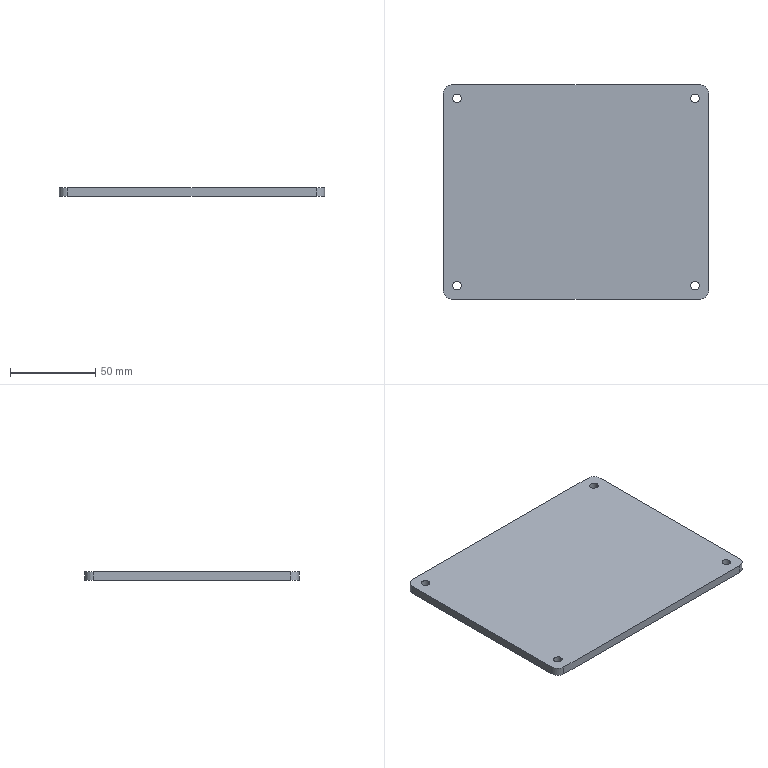Part | STEP file | Wrench controller display guard | 1 solid | 18 faces | box 156 x 126 x 5 mm | volume 97780 mm3 | cylinder 12 | plane 6 | commonest cylinder face diameters 5 x8 10 x4
STEP:
#1=CARTESIAN_POINT('',(0.,0.,0.));
#2=DIRECTION('',(0.,0.,1.));
#3=DIRECTION('',(1.,0.,0.));
#4=AXIS2_PLACEMENT_3D('',#1,#2,#3);
#5=CARTESIAN_POINT('',(67.5,-55.,5.));
#6=VERTEX_POINT('',#5);
#7=CARTESIAN_POINT('',(67.5,-55.,0.));
#8=VERTEX_POINT('',#7);
#9=CARTESIAN_POINT('',(67.5,-55.,5.));
#10=DIRECTION('',(0.,0.,-1.));
#11=VECTOR('',#10,1.);
#12=LINE('',#9,#11);
#13=CARTESIAN_POINT('',(70.,-55.,5.));
#14=DIRECTION('',(0.,0.,-1.));
#15=DIRECTION('',(-1.,0.,0.));
#16=AXIS2_PLACEMENT_3D('',#13,#14,#15);
#17=CYLINDRICAL_SURFACE('',#16,2.5);
#18=CARTESIAN_POINT('',(6.283,0.));
#19=DIRECTION('',(0.,1.));
#20=VECTOR('',#19,1.);
#21=LINE('',#18,#20);
#22=(GEOMETRIC_REPRESENTATION_CONTEXT(2)PARAMETRIC_REPRESENTATION_CONTEXT()REPRESENTATION_CONTEXT('',''));
#23=DEFINITIONAL_REPRESENTATION('',(#21),#22);
#24=PCURVE('',#17,#23);
#25=CARTESIAN_POINT('',(70.,-55.,5.));
#26=DIRECTION('',(0.,0.,-1.));
#27=DIRECTION('',(-1.,0.,0.));
#28=AXIS2_PLACEMENT_3D('',#25,#26,#27);
#29=CYLINDRICAL_SURFACE('',#28,2.5);
#30=CARTESIAN_POINT('',(0.,0.));
#31=DIRECTION('',(0.,1.));
#32=VECTOR('',#31,1.);
#33=LINE('',#30,#32);
#34=(GEOMETRIC_REPRESENTATION_CONTEXT(2)PARAMETRIC_REPRESENTATION_CONTEXT()REPRESENTATION_CONTEXT('',''));
#35=DEFINITIONAL_REPRESENTATION('',(#33),#34);
#36=PCURVE('',#29,#35);
#37=SURFACE_CURVE('',#12,(#24,#36),.PCURVE_S1.);
#38=EDGE_CURVE('',#6,#8,#37,.T.);
#39=ORIENTED_EDGE('',*,*,#38,.T.);
#40=CARTESIAN_POINT('',(72.5,-55.,0.));
#41=VERTEX_POINT('',#40);
#42=CARTESIAN_POINT('',(70.,-55.,0.));
#43=DIRECTION('',(0.,0.,1.));
#44=DIRECTION('',(-1.,0.,0.));
#45=AXIS2_PLACEMENT_3D('',#42,#43,#44);
#46=CIRCLE('',#45,2.5);
#47=CARTESIAN_POINT('',(6.283,5.));
#48=DIRECTION('',(-1.,0.));
#49=VECTOR('',#48,1.);
#50=LINE('',#47,#49);
#51=(GEOMETRIC_REPRESENTATION_CONTEXT(2)PARAMETRIC_REPRESENTATION_CONTEXT()REPRESENTATION_CONTEXT('',''));
#52=DEFINITIONAL_REPRESENTATION('',(#50),#51);
#53=PCURVE('',#17,#52);
#54=CARTESIAN_POINT('',(73.,-58.,0.));
#55=DIRECTION('',(0.,0.,1.));
#56=DIRECTION('',(1.,0.,0.));
#57=AXIS2_PLACEMENT_3D('',#54,#55,#56);
#58=PLANE('',#57);
#59=CARTESIAN_POINT('',(-3.,3.));
#60=DIRECTION('',(-1.,0.));
#61=AXIS2_PLACEMENT_2D('',#59,#60);
#62=CIRCLE('',#61,2.5);
#63=(GEOMETRIC_REPRESENTATION_CONTEXT(2)PARAMETRIC_REPRESENTATION_CONTEXT()REPRESENTATION_CONTEXT('',''));
#64=DEFINITIONAL_REPRESENTATION('',(#62),#63);
#65=PCURVE('',#58,#64);
#66=SURFACE_CURVE('',#46,(#53,#65),.PCURVE_S1.);
#67=EDGE_CURVE('',#8,#41,#66,.T.);
#68=ORIENTED_EDGE('',*,*,#67,.T.);
#69=CARTESIAN_POINT('',(72.5,-55.,5.));
#70=VERTEX_POINT('',#69);
#71=CARTESIAN_POINT('',(72.5,-55.,5.));
#72=DIRECTION('',(0.,0.,-1.));
#73=VECTOR('',#72,1.);
#74=LINE('',#71,#73);
#75=CARTESIAN_POINT('',(3.142,0.));
#76=DIRECTION('',(0.,1.));
#77=VECTOR('',#76,1.);
#78=LINE('',#75,#77);
#79=(GEOMETRIC_REPRESENTATION_CONTEXT(2)PARAMETRIC_REPRESENTATION_CONTEXT()REPRESENTATION_CONTEXT('',''));
#80=DEFINITIONAL_REPRESENTATION('',(#78),#79);
#81=PCURVE('',#17,#80);
#82=CARTESIAN_POINT('',(3.142,0.));
#83=DIRECTION('',(0.,1.));
#84=VECTOR('',#83,1.);
#85=LINE('',#82,#84);
#86=(GEOMETRIC_REPRESENTATION_CONTEXT(2)PARAMETRIC_REPRESENTATION_CONTEXT()REPRESENTATION_CONTEXT('',''));
#87=DEFINITIONAL_REPRESENTATION('',(#85),#86);
#88=PCURVE('',#29,#87);
#89=SURFACE_CURVE('',#74,(#81,#88),.PCURVE_S1.);
#90=EDGE_CURVE('',#70,#41,#89,.T.);
#91=ORIENTED_EDGE('',*,*,#90,.F.);
#92=CARTESIAN_POINT('',(70.,-55.,5.));
#93=DIRECTION('',(0.,0.,-1.));
#94=DIRECTION('',(-1.,0.,0.));
#95=AXIS2_PLACEMENT_3D('',#92,#93,#94);
#96=CIRCLE('',#95,2.5);
#97=CARTESIAN_POINT('',(0.,0.));
#98=DIRECTION('',(1.,0.));
#99=VECTOR('',#98,1.);
#100=LINE('',#97,#99);
#101=(GEOMETRIC_REPRESENTATION_CONTEXT(2)PARAMETRIC_REPRESENTATION_CONTEXT()REPRESENTATION_CONTEXT('',''));
#102=DEFINITIONAL_REPRESENTATION('',(#100),#101);
#103=PCURVE('',#17,#102);
#104=CARTESIAN_POINT('',(73.,-58.,5.));
#105=DIRECTION('',(0.,0.,1.));
#106=DIRECTION('',(1.,0.,0.));
#107=AXIS2_PLACEMENT_3D('',#104,#105,#106);
#108=PLANE('',#107);
#109=CARTESIAN_POINT('',(-5.5,3.));
#110=CARTESIAN_POINT('',(-5.5,7.33));
#111=CARTESIAN_POINT('',(-1.75,5.165));
#112=CARTESIAN_POINT('',(2.,3.));
#113=CARTESIAN_POINT('',(-1.75,0.8349));
#114=CARTESIAN_POINT('',(-5.5,-1.33));
#115=CARTESIAN_POINT('',(-5.5,3.));
#116=(BOUNDED_CURVE()B_SPLINE_CURVE(2,(#109,#110,#111,#112,#113,#114,#115),.UNSPECIFIED.,.T.,.F.)B_SPLINE_CURVE_WITH_KNOTS((1,2,2,2,2,1),(-2.094,0.,2.094,4.189,6.283,8.378),.UNSPECIFIED.)CURVE()GEOMETRIC_REPRESENTATION_ITEM()RATIONAL_B_SPLINE_CURVE((1.,0.5,1.,0.5,1.,0.5,1.))REPRESENTATION_ITEM(''));
#117=(GEOMETRIC_REPRESENTATION_CONTEXT(2)PARAMETRIC_REPRESENTATION_CONTEXT()REPRESENTATION_CONTEXT('',''));
#118=DEFINITIONAL_REPRESENTATION('',(#116),#117);
#119=PCURVE('',#108,#118);
#120=SURFACE_CURVE('',#96,(#103,#119),.PCURVE_S1.);
#121=EDGE_CURVE('',#70,#6,#120,.T.);
#122=ORIENTED_EDGE('',*,*,#121,.T.);
#123=EDGE_LOOP('',(#39,#68,#91,#122));
#124=FACE_BOUND('',#123,.F.);
#125=ADVANCED_FACE('',(#124),#17,.F.);
#126=CARTESIAN_POINT('',(67.5,55.,5.));
#127=VERTEX_POINT('',#126);
#128=CARTESIAN_POINT('',(67.5,55.,0.));
#129=VERTEX_POINT('',#128);
#130=CARTESIAN_POINT('',(67.5,55.,5.));
#131=DIRECTION('',(0.,0.,-1.));
#132=VECTOR('',#131,1.);
#133=LINE('',#130,#132);
#134=CARTESIAN_POINT('',(70.,55.,5.));
#135=DIRECTION('',(0.,0.,-1.));
#136=DIRECTION('',(-1.,0.,0.));
#137=AXIS2_PLACEMENT_3D('',#134,#135,#136);
#138=CYLINDRICAL_SURFACE('',#137,2.5);
#139=CARTESIAN_POINT('',(6.283,0.));
#140=DIRECTION('',(0.,1.));
#141=VECTOR('',#140,1.);
#142=LINE('',#139,#141);
#143=(GEOMETRIC_REPRESENTATION_CONTEXT(2)PARAMETRIC_REPRESENTATION_CONTEXT()REPRESENTATION_CONTEXT('',''));
#144=DEFINITIONAL_REPRESENTATION('',(#142),#143);
#145=PCURVE('',#138,#144);
#146=CARTESIAN_POINT('',(70.,55.,5.));
#147=DIRECTION('',(0.,0.,-1.));
#148=DIRECTION('',(-1.,0.,0.));
#149=AXIS2_PLACEMENT_3D('',#146,#147,#148);
#150=CYLINDRICAL_SURFACE('',#149,2.5);
#151=CARTESIAN_POINT('',(0.,0.));
#152=DIRECTION('',(0.,1.));
#153=VECTOR('',#152,1.);
#154=LINE('',#151,#153);
#155=(GEOMETRIC_REPRESENTATION_CONTEXT(2)PARAMETRIC_REPRESENTATION_CONTEXT()REPRESENTATION_CONTEXT('',''));
#156=DEFINITIONAL_REPRESENTATION('',(#154),#155);
#157=PCURVE('',#150,#156);
#158=SURFACE_CURVE('',#133,(#145,#157),.PCURVE_S1.);
#159=EDGE_CURVE('',#127,#129,#158,.T.);
#160=ORIENTED_EDGE('',*,*,#159,.T.);
#161=CARTESIAN_POINT('',(72.5,55.,0.));
#162=VERTEX_POINT('',#161);
#163=CARTESIAN_POINT('',(70.,55.,0.));
#164=DIRECTION('',(0.,0.,1.));
#165=DIRECTION('',(-1.,0.,0.));
#166=AXIS2_PLACEMENT_3D('',#163,#164,#165);
#167=CIRCLE('',#166,2.5);
#168=CARTESIAN_POINT('',(6.283,5.));
#169=DIRECTION('',(-1.,0.));
#170=VECTOR('',#169,1.);
#171=LINE('',#168,#170);
#172=(GEOMETRIC_REPRESENTATION_CONTEXT(2)PARAMETRIC_REPRESENTATION_CONTEXT()REPRESENTATION_CONTEXT('',''));
#173=DEFINITIONAL_REPRESENTATION('',(#171),#172);
#174=PCURVE('',#138,#173);
#175=CARTESIAN_POINT('',(-3.,113.));
#176=DIRECTION('',(-1.,0.));
#177=AXIS2_PLACEMENT_2D('',#175,#176);
#178=CIRCLE('',#177,2.5);
#179=(GEOMETRIC_REPRESENTATION_CONTEXT(2)PARAMETRIC_REPRESENTATION_CONTEXT()REPRESENTATION_CONTEXT('',''));
#180=DEFINITIONAL_REPRESENTATION('',(#178),#179);
#181=PCURVE('',#58,#180);
#182=SURFACE_CURVE('',#167,(#174,#181),.PCURVE_S1.);
#183=EDGE_CURVE('',#129,#162,#182,.T.);
#184=ORIENTED_EDGE('',*,*,#183,.T.);
#185=CARTESIAN_POINT('',(72.5,55.,5.));
#186=VERTEX_POINT('',#185);
#187=CARTESIAN_POINT('',(72.5,55.,5.));
#188=DIRECTION('',(0.,0.,-1.));
#189=VECTOR('',#188,1.);
#190=LINE('',#187,#189);
#191=CARTESIAN_POINT('',(3.142,0.));
#192=DIRECTION('',(0.,1.));
#193=VECTOR('',#192,1.);
#194=LINE('',#191,#193);
#195=(GEOMETRIC_REPRESENTATION_CONTEXT(2)PARAMETRIC_REPRESENTATION_CONTEXT()REPRESENTATION_CONTEXT('',''));
#196=DEFINITIONAL_REPRESENTATION('',(#194),#195);
#197=PCURVE('',#138,#196);
#198=CARTESIAN_POINT('',(3.142,0.));
#199=DIRECTION('',(0.,1.));
#200=VECTOR('',#199,1.);
#201=LINE('',#198,#200);
#202=(GEOMETRIC_REPRESENTATION_CONTEXT(2)PARAMETRIC_REPRESENTATION_CONTEXT()REPRESENTATION_CONTEXT('',''));
#203=DEFINITIONAL_REPRESENTATION('',(#201),#202);
#204=PCURVE('',#150,#203);
#205=SURFACE_CURVE('',#190,(#197,#204),.PCURVE_S1.);
#206=EDGE_CURVE('',#186,#162,#205,.T.);
#207=ORIENTED_EDGE('',*,*,#206,.F.);
#208=CARTESIAN_POINT('',(70.,55.,5.));
#209=DIRECTION('',(0.,0.,-1.));
#210=DIRECTION('',(-1.,0.,0.));
#211=AXIS2_PLACEMENT_3D('',#208,#209,#210);
#212=CIRCLE('',#211,2.5);
#213=CARTESIAN_POINT('',(0.,0.));
#214=DIRECTION('',(1.,0.));
#215=VECTOR('',#214,1.);
#216=LINE('',#213,#215);
#217=(GEOMETRIC_REPRESENTATION_CONTEXT(2)PARAMETRIC_REPRESENTATION_CONTEXT()REPRESENTATION_CONTEXT('',''));
#218=DEFINITIONAL_REPRESENTATION('',(#216),#217);
#219=PCURVE('',#138,#218);
#220=CARTESIAN_POINT('',(-5.5,113.));
#221=CARTESIAN_POINT('',(-5.5,117.33));
#222=CARTESIAN_POINT('',(-1.75,115.165));
#223=CARTESIAN_POINT('',(2.,113.));
#224=CARTESIAN_POINT('',(-1.75,110.835));
#225=CARTESIAN_POINT('',(-5.5,108.67));
#226=CARTESIAN_POINT('',(-5.5,113.));
#227=(BOUNDED_CURVE()B_SPLINE_CURVE(2,(#220,#221,#222,#223,#224,#225,#226),.UNSPECIFIED.,.T.,.F.)B_SPLINE_CURVE_WITH_KNOTS((1,2,2,2,2,1),(-2.094,0.,2.094,4.189,6.283,8.378),.UNSPECIFIED.)CURVE()GEOMETRIC_REPRESENTATION_ITEM()RATIONAL_B_SPLINE_CURVE((1.,0.5,1.,0.5,1.,0.5,1.))REPRESENTATION_ITEM(''));
#228=(GEOMETRIC_REPRESENTATION_CONTEXT(2)PARAMETRIC_REPRESENTATION_CONTEXT()REPRESENTATION_CONTEXT('',''));
#229=DEFINITIONAL_REPRESENTATION('',(#227),#228);
#230=PCURVE('',#108,#229);
#231=SURFACE_CURVE('',#212,(#219,#230),.PCURVE_S1.);
#232=EDGE_CURVE('',#186,#127,#231,.T.);
#233=ORIENTED_EDGE('',*,*,#232,.T.);
#234=EDGE_LOOP('',(#160,#184,#207,#233));
#235=FACE_BOUND('',#234,.F.);
#236=ADVANCED_FACE('',(#235),#138,.F.);
#237=CARTESIAN_POINT('',(-72.5,55.,5.));
#238=VERTEX_POINT('',#237);
#239=CARTESIAN_POINT('',(-72.5,55.,0.));
#240=VERTEX_POINT('',#239);
#241=CARTESIAN_POINT('',(-72.5,55.,5.));
#242=DIRECTION('',(0.,0.,-1.));
#243=VECTOR('',#242,1.);
#244=LINE('',#241,#243);
#245=CARTESIAN_POINT('',(-70.,55.,5.));
#246=DIRECTION('',(0.,0.,-1.));
#247=DIRECTION('',(-1.,0.,0.));
#248=AXIS2_PLACEMENT_3D('',#245,#246,#247);
#249=CYLINDRICAL_SURFACE('',#248,2.5);
#250=CARTESIAN_POINT('',(6.283,0.));
#251=DIRECTION('',(0.,1.));
#252=VECTOR('',#251,1.);
#253=LINE('',#250,#252);
#254=(GEOMETRIC_REPRESENTATION_CONTEXT(2)PARAMETRIC_REPRESENTATION_CONTEXT()REPRESENTATION_CONTEXT('',''));
#255=DEFINITIONAL_REPRESENTATION('',(#253),#254);
#256=PCURVE('',#249,#255);
#257=CARTESIAN_POINT('',(-70.,55.,5.));
#258=DIRECTION('',(0.,0.,-1.));
#259=DIRECTION('',(-1.,0.,0.));
#260=AXIS2_PLACEMENT_3D('',#257,#258,#259);
#261=CYLINDRICAL_SURFACE('',#260,2.5);
#262=CARTESIAN_POINT('',(0.,0.));
#263=DIRECTION('',(0.,1.));
#264=VECTOR('',#263,1.);
#265=LINE('',#262,#264);
#266=(GEOMETRIC_REPRESENTATION_CONTEXT(2)PARAMETRIC_REPRESENTATION_CONTEXT()REPRESENTATION_CONTEXT('',''));
#267=DEFINITIONAL_REPRESENTATION('',(#265),#266);
#268=PCURVE('',#261,#267);
#269=SURFACE_CURVE('',#244,(#256,#268),.PCURVE_S1.);
#270=EDGE_CURVE('',#238,#240,#269,.T.);
#271=ORIENTED_EDGE('',*,*,#270,.T.);
#272=CARTESIAN_POINT('',(-67.5,55.,0.));
#273=VERTEX_POINT('',#272);
#274=CARTESIAN_POINT('',(-70.,55.,0.));
#275=DIRECTION('',(0.,0.,1.));
#276=DIRECTION('',(-1.,0.,0.));
#277=AXIS2_PLACEMENT_3D('',#274,#275,#276);
#278=CIRCLE('',#277,2.5);
#279=CARTESIAN_POINT('',(6.283,5.));
#280=DIRECTION('',(-1.,0.));
#281=VECTOR('',#280,1.);
#282=LINE('',#279,#281);
#283=(GEOMETRIC_REPRESENTATION_CONTEXT(2)PARAMETRIC_REPRESENTATION_CONTEXT()REPRESENTATION_CONTEXT('',''));
#284=DEFINITIONAL_REPRESENTATION('',(#282),#283);
#285=PCURVE('',#249,#284);
#286=CARTESIAN_POINT('',(-143.,113.));
#287=DIRECTION('',(-1.,0.));
#288=AXIS2_PLACEMENT_2D('',#286,#287);
#289=CIRCLE('',#288,2.5);
#290=(GEOMETRIC_REPRESENTATION_CONTEXT(2)PARAMETRIC_REPRESENTATION_CONTEXT()REPRESENTATION_CONTEXT('',''));
#291=DEFINITIONAL_REPRESENTATION('',(#289),#290);
#292=PCURVE('',#58,#291);
#293=SURFACE_CURVE('',#278,(#285,#292),.PCURVE_S1.);
#294=EDGE_CURVE('',#240,#273,#293,.T.);
#295=ORIENTED_EDGE('',*,*,#294,.T.);
#296=CARTESIAN_POINT('',(-67.5,55.,5.));
#297=VERTEX_POINT('',#296);
#298=CARTESIAN_POINT('',(-67.5,55.,5.));
#299=DIRECTION('',(0.,0.,-1.));
#300=VECTOR('',#299,1.);
#301=LINE('',#298,#300);
#302=CARTESIAN_POINT('',(3.142,0.));
#303=DIRECTION('',(0.,1.));
#304=VECTOR('',#303,1.);
#305=LINE('',#302,#304);
#306=(GEOMETRIC_REPRESENTATION_CONTEXT(2)PARAMETRIC_REPRESENTATION_CONTEXT()REPRESENTATION_CONTEXT('',''));
#307=DEFINITIONAL_REPRESENTATION('',(#305),#306);
#308=PCURVE('',#249,#307);
#309=CARTESIAN_POINT('',(3.142,0.));
#310=DIRECTION('',(0.,1.));
#311=VECTOR('',#310,1.);
#312=LINE('',#309,#311);
#313=(GEOMETRIC_REPRESENTATION_CONTEXT(2)PARAMETRIC_REPRESENTATION_CONTEXT()REPRESENTATION_CONTEXT('',''));
#314=DEFINITIONAL_REPRESENTATION('',(#312),#313);
#315=PCURVE('',#261,#314);
#316=SURFACE_CURVE('',#301,(#308,#315),.PCURVE_S1.);
#317=EDGE_CURVE('',#297,#273,#316,.T.);
#318=ORIENTED_EDGE('',*,*,#317,.F.);
#319=CARTESIAN_POINT('',(-70.,55.,5.));
#320=DIRECTION('',(0.,0.,-1.));
#321=DIRECTION('',(-1.,0.,0.));
#322=AXIS2_PLACEMENT_3D('',#319,#320,#321);
#323=CIRCLE('',#322,2.5);
#324=CARTESIAN_POINT('',(0.,0.));
#325=DIRECTION('',(1.,0.));
#326=VECTOR('',#325,1.);
#327=LINE('',#324,#326);
#328=(GEOMETRIC_REPRESENTATION_CONTEXT(2)PARAMETRIC_REPRESENTATION_CONTEXT()REPRESENTATION_CONTEXT('',''));
#329=DEFINITIONAL_REPRESENTATION('',(#327),#328);
#330=PCURVE('',#249,#329);
#331=CARTESIAN_POINT('',(-145.5,113.));
#332=CARTESIAN_POINT('',(-145.5,117.33));
#333=CARTESIAN_POINT('',(-141.75,115.165));
#334=CARTESIAN_POINT('',(-138.,113.));
#335=CARTESIAN_POINT('',(-141.75,110.835));
#336=CARTESIAN_POINT('',(-145.5,108.67));
#337=CARTESIAN_POINT('',(-145.5,113.));
#338=(BOUNDED_CURVE()B_SPLINE_CURVE(2,(#331,#332,#333,#334,#335,#336,#337),.UNSPECIFIED.,.T.,.F.)B_SPLINE_CURVE_WITH_KNOTS((1,2,2,2,2,1),(-2.094,0.,2.094,4.189,6.283,8.378),.UNSPECIFIED.)CURVE()GEOMETRIC_REPRESENTATION_ITEM()RATIONAL_B_SPLINE_CURVE((1.,0.5,1.,0.5,1.,0.5,1.))REPRESENTATION_ITEM(''));
#339=(GEOMETRIC_REPRESENTATION_CONTEXT(2)PARAMETRIC_REPRESENTATION_CONTEXT()REPRESENTATION_CONTEXT('',''));
#340=DEFINITIONAL_REPRESENTATION('',(#338),#339);
#341=PCURVE('',#108,#340);
#342=SURFACE_CURVE('',#323,(#330,#341),.PCURVE_S1.);
#343=EDGE_CURVE('',#297,#238,#342,.T.);
#344=ORIENTED_EDGE('',*,*,#343,.T.);
#345=EDGE_LOOP('',(#271,#295,#318,#344));
#346=FACE_BOUND('',#345,.F.);
#347=ADVANCED_FACE('',(#346),#249,.F.);
#348=CARTESIAN_POINT('',(-72.5,-55.,5.));
#349=VERTEX_POINT('',#348);
#350=CARTESIAN_POINT('',(-72.5,-55.,0.));
#351=VERTEX_POINT('',#350);
#352=CARTESIAN_POINT('',(-72.5,-55.,5.));
#353=DIRECTION('',(0.,0.,-1.));
#354=VECTOR('',#353,1.);
#355=LINE('',#352,#354);
#356=CARTESIAN_POINT('',(-70.,-55.,5.));
#357=DIRECTION('',(0.,0.,-1.));
#358=DIRECTION('',(-1.,0.,0.));
#359=AXIS2_PLACEMENT_3D('',#356,#357,#358);
#360=CYLINDRICAL_SURFACE('',#359,2.5);
#361=CARTESIAN_POINT('',(6.283,0.));
#362=DIRECTION('',(0.,1.));
#363=VECTOR('',#362,1.);
#364=LINE('',#361,#363);
#365=(GEOMETRIC_REPRESENTATION_CONTEXT(2)PARAMETRIC_REPRESENTATION_CONTEXT()REPRESENTATION_CONTEXT('',''));
#366=DEFINITIONAL_REPRESENTATION('',(#364),#365);
#367=PCURVE('',#360,#366);
#368=CARTESIAN_POINT('',(-70.,-55.,5.));
#369=DIRECTION('',(0.,0.,-1.));
#370=DIRECTION('',(-1.,0.,0.));
#371=AXIS2_PLACEMENT_3D('',#368,#369,#370);
#372=CYLINDRICAL_SURFACE('',#371,2.5);
#373=CARTESIAN_POINT('',(0.,0.));
#374=DIRECTION('',(0.,1.));
#375=VECTOR('',#374,1.);
#376=LINE('',#373,#375);
#377=(GEOMETRIC_REPRESENTATION_CONTEXT(2)PARAMETRIC_REPRESENTATION_CONTEXT()REPRESENTATION_CONTEXT('',''));
#378=DEFINITIONAL_REPRESENTATION('',(#376),#377);
#379=PCURVE('',#372,#378);
#380=SURFACE_CURVE('',#355,(#367,#379),.PCURVE_S1.);
#381=EDGE_CURVE('',#349,#351,#380,.T.);
#382=ORIENTED_EDGE('',*,*,#381,.T.);
#383=CARTESIAN_POINT('',(-67.5,-55.,0.));
#384=VERTEX_POINT('',#383);
#385=CARTESIAN_POINT('',(-70.,-55.,0.));
#386=DIRECTION('',(0.,0.,1.));
#387=DIRECTION('',(-1.,0.,0.));
#388=AXIS2_PLACEMENT_3D('',#385,#386,#387);
#389=CIRCLE('',#388,2.5);
#390=CARTESIAN_POINT('',(6.283,5.));
#391=DIRECTION('',(-1.,0.));
#392=VECTOR('',#391,1.);
#393=LINE('',#390,#392);
#394=(GEOMETRIC_REPRESENTATION_CONTEXT(2)PARAMETRIC_REPRESENTATION_CONTEXT()REPRESENTATION_CONTEXT('',''));
#395=DEFINITIONAL_REPRESENTATION('',(#393),#394);
#396=PCURVE('',#360,#395);
#397=CARTESIAN_POINT('',(-143.,3.));
#398=DIRECTION('',(-1.,0.));
#399=AXIS2_PLACEMENT_2D('',#397,#398);
#400=CIRCLE('',#399,2.5);
#401=(GEOMETRIC_REPRESENTATION_CONTEXT(2)PARAMETRIC_REPRESENTATION_CONTEXT()REPRESENTATION_CONTEXT('',''));
#402=DEFINITIONAL_REPRESENTATION('',(#400),#401);
#403=PCURVE('',#58,#402);
#404=SURFACE_CURVE('',#389,(#396,#403),.PCURVE_S1.);
#405=EDGE_CURVE('',#351,#384,#404,.T.);
#406=ORIENTED_EDGE('',*,*,#405,.T.);
#407=CARTESIAN_POINT('',(-67.5,-55.,5.));
#408=VERTEX_POINT('',#407);
#409=CARTESIAN_POINT('',(-67.5,-55.,5.));
#410=DIRECTION('',(0.,0.,-1.));
#411=VECTOR('',#410,1.);
#412=LINE('',#409,#411);
#413=CARTESIAN_POINT('',(3.142,0.));
#414=DIRECTION('',(0.,1.));
#415=VECTOR('',#414,1.);
#416=LINE('',#413,#415);
#417=(GEOMETRIC_REPRESENTATION_CONTEXT(2)PARAMETRIC_REPRESENTATION_CONTEXT()REPRESENTATION_CONTEXT('',''));
#418=DEFINITIONAL_REPRESENTATION('',(#416),#417);
#419=PCURVE('',#360,#418);
#420=CARTESIAN_POINT('',(3.142,0.));
#421=DIRECTION('',(0.,1.));
#422=VECTOR('',#421,1.);
#423=LINE('',#420,#422);
#424=(GEOMETRIC_REPRESENTATION_CONTEXT(2)PARAMETRIC_REPRESENTATION_CONTEXT()REPRESENTATION_CONTEXT('',''));
#425=DEFINITIONAL_REPRESENTATION('',(#423),#424);
#426=PCURVE('',#372,#425);
#427=SURFACE_CURVE('',#412,(#419,#426),.PCURVE_S1.);
#428=EDGE_CURVE('',#408,#384,#427,.T.);
#429=ORIENTED_EDGE('',*,*,#428,.F.);
#430=CARTESIAN_POINT('',(-70.,-55.,5.));
#431=DIRECTION('',(0.,0.,-1.));
#432=DIRECTION('',(-1.,0.,0.));
#433=AXIS2_PLACEMENT_3D('',#430,#431,#432);
#434=CIRCLE('',#433,2.5);
#435=CARTESIAN_POINT('',(0.,0.));
#436=DIRECTION('',(1.,0.));
#437=VECTOR('',#436,1.);
#438=LINE('',#435,#437);
#439=(GEOMETRIC_REPRESENTATION_CONTEXT(2)PARAMETRIC_REPRESENTATION_CONTEXT()REPRESENTATION_CONTEXT('',''));
#440=DEFINITIONAL_REPRESENTATION('',(#438),#439);
#441=PCURVE('',#360,#440);
#442=CARTESIAN_POINT('',(-145.5,3.));
#443=CARTESIAN_POINT('',(-145.5,7.33));
#444=CARTESIAN_POINT('',(-141.75,5.165));
#445=CARTESIAN_POINT('',(-138.,3.));
#446=CARTESIAN_POINT('',(-141.75,0.8349));
#447=CARTESIAN_POINT('',(-145.5,-1.33));
#448=CARTESIAN_POINT('',(-145.5,3.));
#449=(BOUNDED_CURVE()B_SPLINE_CURVE(2,(#442,#443,#444,#445,#446,#447,#448),.UNSPECIFIED.,.T.,.F.)B_SPLINE_CURVE_WITH_KNOTS((1,2,2,2,2,1),(-2.094,0.,2.094,4.189,6.283,8.378),.UNSPECIFIED.)CURVE()GEOMETRIC_REPRESENTATION_ITEM()RATIONAL_B_SPLINE_CURVE((1.,0.5,1.,0.5,1.,0.5,1.))REPRESENTATION_ITEM(''));
#450=(GEOMETRIC_REPRESENTATION_CONTEXT(2)PARAMETRIC_REPRESENTATION_CONTEXT()REPRESENTATION_CONTEXT('',''));
#451=DEFINITIONAL_REPRESENTATION('',(#449),#450);
#452=PCURVE('',#108,#451);
#453=SURFACE_CURVE('',#434,(#441,#452),.PCURVE_S1.);
#454=EDGE_CURVE('',#408,#349,#453,.T.);
#455=ORIENTED_EDGE('',*,*,#454,.T.);
#456=EDGE_LOOP('',(#382,#406,#429,#455));
#457=FACE_BOUND('',#456,.F.);
#458=ADVANCED_FACE('',(#457),#360,.F.);
#459=CARTESIAN_POINT('',(70.,-55.,5.));
#460=DIRECTION('',(0.,0.,-1.));
#461=DIRECTION('',(-1.,0.,0.));
#462=AXIS2_PLACEMENT_3D('',#459,#460,#461);
#463=CIRCLE('',#462,2.5);
#464=CARTESIAN_POINT('',(-5.5,3.));
#465=CARTESIAN_POINT('',(-5.5,7.33));
#466=CARTESIAN_POINT('',(-1.75,5.165));
#467=CARTESIAN_POINT('',(2.,3.));
#468=CARTESIAN_POINT('',(-1.75,0.8349));
#469=CARTESIAN_POINT('',(-5.5,-1.33));
#470=CARTESIAN_POINT('',(-5.5,3.));
#471=(BOUNDED_CURVE()B_SPLINE_CURVE(2,(#464,#465,#466,#467,#468,#469,#470),.UNSPECIFIED.,.T.,.F.)B_SPLINE_CURVE_WITH_KNOTS((1,2,2,2,2,1),(-2.094,0.,2.094,4.189,6.283,8.378),.UNSPECIFIED.)CURVE()GEOMETRIC_REPRESENTATION_ITEM()RATIONAL_B_SPLINE_CURVE((1.,0.5,1.,0.5,1.,0.5,1.))REPRESENTATION_ITEM(''));
#472=(GEOMETRIC_REPRESENTATION_CONTEXT(2)PARAMETRIC_REPRESENTATION_CONTEXT()REPRESENTATION_CONTEXT('',''));
#473=DEFINITIONAL_REPRESENTATION('',(#471),#472);
#474=PCURVE('',#108,#473);
#475=CARTESIAN_POINT('',(0.,0.));
#476=DIRECTION('',(1.,0.));
#477=VECTOR('',#476,1.);
#478=LINE('',#475,#477);
#479=(GEOMETRIC_REPRESENTATION_CONTEXT(2)PARAMETRIC_REPRESENTATION_CONTEXT()REPRESENTATION_CONTEXT('',''));
#480=DEFINITIONAL_REPRESENTATION('',(#478),#479);
#481=PCURVE('',#29,#480);
#482=SURFACE_CURVE('',#463,(#474,#481),.PCURVE_S1.);
#483=EDGE_CURVE('',#6,#70,#482,.T.);
#484=ORIENTED_EDGE('',*,*,#483,.T.);
#485=ORIENTED_EDGE('',*,*,#121,.T.);
#486=EDGE_LOOP('',(#484,#485));
#487=FACE_BOUND('',#486,.T.);
#488=CARTESIAN_POINT('',(70.,55.,5.));
#489=DIRECTION('',(0.,0.,-1.));
#490=DIRECTION('',(-1.,0.,0.));
#491=AXIS2_PLACEMENT_3D('',#488,#489,#490);
#492=CIRCLE('',#491,2.5);
#493=CARTESIAN_POINT('',(-5.5,113.));
#494=CARTESIAN_POINT('',(-5.5,117.33));
#495=CARTESIAN_POINT('',(-1.75,115.165));
#496=CARTESIAN_POINT('',(2.,113.));
#497=CARTESIAN_POINT('',(-1.75,110.835));
#498=CARTESIAN_POINT('',(-5.5,108.67));
#499=CARTESIAN_POINT('',(-5.5,113.));
#500=(BOUNDED_CURVE()B_SPLINE_CURVE(2,(#493,#494,#495,#496,#497,#498,#499),.UNSPECIFIED.,.T.,.F.)B_SPLINE_CURVE_WITH_KNOTS((1,2,2,2,2,1),(-2.094,0.,2.094,4.189,6.283,8.378),.UNSPECIFIED.)CURVE()GEOMETRIC_REPRESENTATION_ITEM()RATIONAL_B_SPLINE_CURVE((1.,0.5,1.,0.5,1.,0.5,1.))REPRESENTATION_ITEM(''));
#501=(GEOMETRIC_REPRESENTATION_CONTEXT(2)PARAMETRIC_REPRESENTATION_CONTEXT()REPRESENTATION_CONTEXT('',''));
#502=DEFINITIONAL_REPRESENTATION('',(#500),#501);
#503=PCURVE('',#108,#502);
#504=CARTESIAN_POINT('',(0.,0.));
#505=DIRECTION('',(1.,0.));
#506=VECTOR('',#505,1.);
#507=LINE('',#504,#506);
#508=(GEOMETRIC_REPRESENTATION_CONTEXT(2)PARAMETRIC_REPRESENTATION_CONTEXT()REPRESENTATION_CONTEXT('',''));
#509=DEFINITIONAL_REPRESENTATION('',(#507),#508);
#510=PCURVE('',#150,#509);
#511=SURFACE_CURVE('',#492,(#503,#510),.PCURVE_S1.);
#512=EDGE_CURVE('',#127,#186,#511,.T.);
#513=ORIENTED_EDGE('',*,*,#512,.T.);
#514=ORIENTED_EDGE('',*,*,#232,.T.);
#515=EDGE_LOOP('',(#513,#514));
#516=FACE_BOUND('',#515,.T.);
#517=CARTESIAN_POINT('',(-78.,-58.,5.));
#518=VERTEX_POINT('',#517);
#519=CARTESIAN_POINT('',(-73.,-63.,5.));
#520=VERTEX_POINT('',#519);
#521=CARTESIAN_POINT('',(-73.,-58.,5.));
#522=DIRECTION('',(0.,0.,1.));
#523=DIRECTION('',(-1.,0.,0.));
#524=AXIS2_PLACEMENT_3D('',#521,#522,#523);
#525=CIRCLE('',#524,5.);
#526=CARTESIAN_POINT('',(-146.,0.));
#527=DIRECTION('',(-1.,0.));
#528=AXIS2_PLACEMENT_2D('',#526,#527);
#529=CIRCLE('',#528,5.);
#530=(GEOMETRIC_REPRESENTATION_CONTEXT(2)PARAMETRIC_REPRESENTATION_CONTEXT()REPRESENTATION_CONTEXT('',''));
#531=DEFINITIONAL_REPRESENTATION('',(#529),#530);
#532=PCURVE('',#108,#531);
#533=CARTESIAN_POINT('',(-73.,-58.,5.));
#534=DIRECTION('',(0.,0.,-1.));
#535=DIRECTION('',(-1.,0.,0.));
#536=AXIS2_PLACEMENT_3D('',#533,#534,#535);
#537=CYLINDRICAL_SURFACE('',#536,5.);
#538=CARTESIAN_POINT('',(6.283,0.));
#539=DIRECTION('',(-1.,0.));
#540=VECTOR('',#539,1.);
#541=LINE('',#538,#540);
#542=(GEOMETRIC_REPRESENTATION_CONTEXT(2)PARAMETRIC_REPRESENTATION_CONTEXT()REPRESENTATION_CONTEXT('',''));
#543=DEFINITIONAL_REPRESENTATION('',(#541),#542);
#544=PCURVE('',#537,#543);
#545=SURFACE_CURVE('',#525,(#532,#544),.PCURVE_S1.);
#546=EDGE_CURVE('',#518,#520,#545,.T.);
#547=ORIENTED_EDGE('',*,*,#546,.T.);
#548=CARTESIAN_POINT('',(73.,-63.,5.));
#549=VERTEX_POINT('',#548);
#550=CARTESIAN_POINT('',(73.,-63.,5.));
#551=DIRECTION('',(1.,0.,0.));
#552=VECTOR('',#551,1.);
#553=LINE('',#550,#552);
#554=CARTESIAN_POINT('',(0.,-5.));
#555=DIRECTION('',(1.,0.));
#556=VECTOR('',#555,1.);
#557=LINE('',#554,#556);
#558=(GEOMETRIC_REPRESENTATION_CONTEXT(2)PARAMETRIC_REPRESENTATION_CONTEXT()REPRESENTATION_CONTEXT('',''));
#559=DEFINITIONAL_REPRESENTATION('',(#557),#558);
#560=PCURVE('',#108,#559);
#561=CARTESIAN_POINT('',(-73.,-63.,5.));
#562=DIRECTION('',(0.,1.,0.));
#563=DIRECTION('',(-1.,0.,0.));
#564=AXIS2_PLACEMENT_3D('',#561,#562,#563);
#565=PLANE('',#564);
#566=CARTESIAN_POINT('',(-146.,0.));
#567=DIRECTION('',(-1.,0.));
#568=VECTOR('',#567,1.);
#569=LINE('',#566,#568);
#570=(GEOMETRIC_REPRESENTATION_CONTEXT(2)PARAMETRIC_REPRESENTATION_CONTEXT()REPRESENTATION_CONTEXT('',''));
#571=DEFINITIONAL_REPRESENTATION('',(#569),#570);
#572=PCURVE('',#565,#571);
#573=SURFACE_CURVE('',#553,(#560,#572),.PCURVE_S1.);
#574=EDGE_CURVE('',#520,#549,#573,.T.);
#575=ORIENTED_EDGE('',*,*,#574,.T.);
#576=CARTESIAN_POINT('',(78.,-58.,5.));
#577=VERTEX_POINT('',#576);
#578=CARTESIAN_POINT('',(73.,-58.,5.));
#579=DIRECTION('',(0.,0.,1.));
#580=DIRECTION('',(-1.,0.,0.));
#581=AXIS2_PLACEMENT_3D('',#578,#579,#580);
#582=CIRCLE('',#581,5.);
#583=CARTESIAN_POINT('',(0.,0.));
#584=DIRECTION('',(-1.,0.));
#585=AXIS2_PLACEMENT_2D('',#583,#584);
#586=CIRCLE('',#585,5.);
#587=(GEOMETRIC_REPRESENTATION_CONTEXT(2)PARAMETRIC_REPRESENTATION_CONTEXT()REPRESENTATION_CONTEXT('',''));
#588=DEFINITIONAL_REPRESENTATION('',(#586),#587);
#589=PCURVE('',#108,#588);
#590=CARTESIAN_POINT('',(73.,-58.,5.));
#591=DIRECTION('',(0.,0.,-1.));
#592=DIRECTION('',(-1.,0.,0.));
#593=AXIS2_PLACEMENT_3D('',#590,#591,#592);
#594=CYLINDRICAL_SURFACE('',#593,5.);
#595=CARTESIAN_POINT('',(6.283,0.));
#596=DIRECTION('',(-1.,0.));
#597=VECTOR('',#596,1.);
#598=LINE('',#595,#597);
#599=(GEOMETRIC_REPRESENTATION_CONTEXT(2)PARAMETRIC_REPRESENTATION_CONTEXT()REPRESENTATION_CONTEXT('',''));
#600=DEFINITIONAL_REPRESENTATION('',(#598),#599);
#601=PCURVE('',#594,#600);
#602=SURFACE_CURVE('',#582,(#589,#601),.PCURVE_S1.);
#603=EDGE_CURVE('',#549,#577,#602,.T.);
#604=ORIENTED_EDGE('',*,*,#603,.T.);
#605=CARTESIAN_POINT('',(78.,58.,5.));
#606=VERTEX_POINT('',#605);
#607=CARTESIAN_POINT('',(78.,-58.,5.));
#608=DIRECTION('',(0.,1.,0.));
#609=VECTOR('',#608,1.);
#610=LINE('',#607,#609);
#611=CARTESIAN_POINT('',(5.,0.));
#612=DIRECTION('',(0.,1.));
#613=VECTOR('',#612,1.);
#614=LINE('',#611,#613);
#615=(GEOMETRIC_REPRESENTATION_CONTEXT(2)PARAMETRIC_REPRESENTATION_CONTEXT()REPRESENTATION_CONTEXT('',''));
#616=DEFINITIONAL_REPRESENTATION('',(#614),#615);
#617=PCURVE('',#108,#616);
#618=CARTESIAN_POINT('',(78.,58.,5.));
#619=DIRECTION('',(-1.,0.,0.));
#620=DIRECTION('',(0.,-1.,0.));
#621=AXIS2_PLACEMENT_3D('',#618,#619,#620);
#622=PLANE('',#621);
#623=CARTESIAN_POINT('',(116.,0.));
#624=DIRECTION('',(-1.,0.));
#625=VECTOR('',#624,1.);
#626=LINE('',#623,#625);
#627=(GEOMETRIC_REPRESENTATION_CONTEXT(2)PARAMETRIC_REPRESENTATION_CONTEXT()REPRESENTATION_CONTEXT('',''));
#628=DEFINITIONAL_REPRESENTATION('',(#626),#627);
#629=PCURVE('',#622,#628);
#630=SURFACE_CURVE('',#610,(#617,#629),.PCURVE_S1.);
#631=EDGE_CURVE('',#577,#606,#630,.T.);
#632=ORIENTED_EDGE('',*,*,#631,.T.);
#633=CARTESIAN_POINT('',(73.,63.,5.));
#634=VERTEX_POINT('',#633);
#635=CARTESIAN_POINT('',(73.,58.,5.));
#636=DIRECTION('',(0.,0.,1.));
#637=DIRECTION('',(-1.,0.,0.));
#638=AXIS2_PLACEMENT_3D('',#635,#636,#637);
#639=CIRCLE('',#638,5.);
#640=CARTESIAN_POINT('',(0.,116.));
#641=DIRECTION('',(-1.,0.));
#642=AXIS2_PLACEMENT_2D('',#640,#641);
#643=CIRCLE('',#642,5.);
#644=(GEOMETRIC_REPRESENTATION_CONTEXT(2)PARAMETRIC_REPRESENTATION_CONTEXT()REPRESENTATION_CONTEXT('',''));
#645=DEFINITIONAL_REPRESENTATION('',(#643),#644);
#646=PCURVE('',#108,#645);
#647=CARTESIAN_POINT('',(73.,58.,5.));
#648=DIRECTION('',(0.,0.,-1.));
#649=DIRECTION('',(-1.,0.,0.));
#650=AXIS2_PLACEMENT_3D('',#647,#648,#649);
#651=CYLINDRICAL_SURFACE('',#650,5.);
#652=CARTESIAN_POINT('',(6.283,0.));
#653=DIRECTION('',(-1.,0.));
#654=VECTOR('',#653,1.);
#655=LINE('',#652,#654);
#656=(GEOMETRIC_REPRESENTATION_CONTEXT(2)PARAMETRIC_REPRESENTATION_CONTEXT()REPRESENTATION_CONTEXT('',''));
#657=DEFINITIONAL_REPRESENTATION('',(#655),#656);
#658=PCURVE('',#651,#657);
#659=SURFACE_CURVE('',#639,(#646,#658),.PCURVE_S1.);
#660=EDGE_CURVE('',#606,#634,#659,.T.);
#661=ORIENTED_EDGE('',*,*,#660,.T.);
#662=CARTESIAN_POINT('',(-73.,63.,5.));
#663=VERTEX_POINT('',#662);
#664=CARTESIAN_POINT('',(73.,63.,5.));
#665=DIRECTION('',(-1.,0.,0.));
#666=VECTOR('',#665,1.);
#667=LINE('',#664,#666);
#668=CARTESIAN_POINT('',(0.,121.));
#669=DIRECTION('',(-1.,0.));
#670=VECTOR('',#669,1.);
#671=LINE('',#668,#670);
#672=(GEOMETRIC_REPRESENTATION_CONTEXT(2)PARAMETRIC_REPRESENTATION_CONTEXT()REPRESENTATION_CONTEXT('',''));
#673=DEFINITIONAL_REPRESENTATION('',(#671),#672);
#674=PCURVE('',#108,#673);
#675=CARTESIAN_POINT('',(-73.,63.,5.));
#676=DIRECTION('',(0.,-1.,0.));
#677=DIRECTION('',(1.,0.,0.));
#678=AXIS2_PLACEMENT_3D('',#675,#676,#677);
#679=PLANE('',#678);
#680=CARTESIAN_POINT('',(146.,0.));
#681=DIRECTION('',(-1.,0.));
#682=VECTOR('',#681,1.);
#683=LINE('',#680,#682);
#684=(GEOMETRIC_REPRESENTATION_CONTEXT(2)PARAMETRIC_REPRESENTATION_CONTEXT()REPRESENTATION_CONTEXT('',''));
#685=DEFINITIONAL_REPRESENTATION('',(#683),#684);
#686=PCURVE('',#679,#685);
#687=SURFACE_CURVE('',#667,(#674,#686),.PCURVE_S1.);
#688=EDGE_CURVE('',#634,#663,#687,.T.);
#689=ORIENTED_EDGE('',*,*,#688,.T.);
#690=CARTESIAN_POINT('',(-78.,58.,5.));
#691=VERTEX_POINT('',#690);
#692=CARTESIAN_POINT('',(-73.,58.,5.));
#693=DIRECTION('',(0.,0.,1.));
#694=DIRECTION('',(-1.,0.,0.));
#695=AXIS2_PLACEMENT_3D('',#692,#693,#694);
#696=CIRCLE('',#695,5.);
#697=CARTESIAN_POINT('',(-146.,116.));
#698=DIRECTION('',(-1.,0.));
#699=AXIS2_PLACEMENT_2D('',#697,#698);
#700=CIRCLE('',#699,5.);
#701=(GEOMETRIC_REPRESENTATION_CONTEXT(2)PARAMETRIC_REPRESENTATION_CONTEXT()REPRESENTATION_CONTEXT('',''));
#702=DEFINITIONAL_REPRESENTATION('',(#700),#701);
#703=PCURVE('',#108,#702);
#704=CARTESIAN_POINT('',(-73.,58.,5.));
#705=DIRECTION('',(0.,0.,-1.));
#706=DIRECTION('',(-1.,0.,0.));
#707=AXIS2_PLACEMENT_3D('',#704,#705,#706);
#708=CYLINDRICAL_SURFACE('',#707,5.);
#709=CARTESIAN_POINT('',(6.283,0.));
#710=DIRECTION('',(-1.,0.));
#711=VECTOR('',#710,1.);
#712=LINE('',#709,#711);
#713=(GEOMETRIC_REPRESENTATION_CONTEXT(2)PARAMETRIC_REPRESENTATION_CONTEXT()REPRESENTATION_CONTEXT('',''));
#714=DEFINITIONAL_REPRESENTATION('',(#712),#713);
#715=PCURVE('',#708,#714);
#716=SURFACE_CURVE('',#696,(#703,#715),.PCURVE_S1.);
#717=EDGE_CURVE('',#663,#691,#716,.T.);
#718=ORIENTED_EDGE('',*,*,#717,.T.);
#719=CARTESIAN_POINT('',(-78.,-58.,5.));
#720=DIRECTION('',(0.,-1.,0.));
#721=VECTOR('',#720,1.);
#722=LINE('',#719,#721);
#723=CARTESIAN_POINT('',(-151.,0.));
#724=DIRECTION('',(0.,-1.));
#725=VECTOR('',#724,1.);
#726=LINE('',#723,#725);
#727=(GEOMETRIC_REPRESENTATION_CONTEXT(2)PARAMETRIC_REPRESENTATION_CONTEXT()REPRESENTATION_CONTEXT('',''));
#728=DEFINITIONAL_REPRESENTATION('',(#726),#727);
#729=PCURVE('',#108,#728);
#730=CARTESIAN_POINT('',(-78.,58.,5.));
#731=DIRECTION('',(1.,0.,0.));
#732=DIRECTION('',(0.,1.,0.));
#733=AXIS2_PLACEMENT_3D('',#730,#731,#732);
#734=PLANE('',#733);
#735=CARTESIAN_POINT('',(-116.,0.));
#736=DIRECTION('',(-1.,0.));
#737=VECTOR('',#736,1.);
#738=LINE('',#735,#737);
#739=(GEOMETRIC_REPRESENTATION_CONTEXT(2)PARAMETRIC_REPRESENTATION_CONTEXT()REPRESENTATION_CONTEXT('',''));
#740=DEFINITIONAL_REPRESENTATION('',(#738),#739);
#741=PCURVE('',#734,#740);
#742=SURFACE_CURVE('',#722,(#729,#741),.PCURVE_S1.);
#743=EDGE_CURVE('',#691,#518,#742,.T.);
#744=ORIENTED_EDGE('',*,*,#743,.T.);
#745=EDGE_LOOP('',(#547,#575,#604,#632,#661,#689,#718,#744));
#746=FACE_BOUND('',#745,.T.);
#747=CARTESIAN_POINT('',(-70.,55.,5.));
#748=DIRECTION('',(0.,0.,-1.));
#749=DIRECTION('',(-1.,0.,0.));
#750=AXIS2_PLACEMENT_3D('',#747,#748,#749);
#751=CIRCLE('',#750,2.5);
#752=CARTESIAN_POINT('',(-145.5,113.));
#753=CARTESIAN_POINT('',(-145.5,117.33));
#754=CARTESIAN_POINT('',(-141.75,115.165));
#755=CARTESIAN_POINT('',(-138.,113.));
#756=CARTESIAN_POINT('',(-141.75,110.835));
#757=CARTESIAN_POINT('',(-145.5,108.67));
#758=CARTESIAN_POINT('',(-145.5,113.));
#759=(BOUNDED_CURVE()B_SPLINE_CURVE(2,(#752,#753,#754,#755,#756,#757,#758),.UNSPECIFIED.,.T.,.F.)B_SPLINE_CURVE_WITH_KNOTS((1,2,2,2,2,1),(-2.094,0.,2.094,4.189,6.283,8.378),.UNSPECIFIED.)CURVE()GEOMETRIC_REPRESENTATION_ITEM()RATIONAL_B_SPLINE_CURVE((1.,0.5,1.,0.5,1.,0.5,1.))REPRESENTATION_ITEM(''));
#760=(GEOMETRIC_REPRESENTATION_CONTEXT(2)PARAMETRIC_REPRESENTATION_CONTEXT()REPRESENTATION_CONTEXT('',''));
#761=DEFINITIONAL_REPRESENTATION('',(#759),#760);
#762=PCURVE('',#108,#761);
#763=CARTESIAN_POINT('',(0.,0.));
#764=DIRECTION('',(1.,0.));
#765=VECTOR('',#764,1.);
#766=LINE('',#763,#765);
#767=(GEOMETRIC_REPRESENTATION_CONTEXT(2)PARAMETRIC_REPRESENTATION_CONTEXT()REPRESENTATION_CONTEXT('',''));
#768=DEFINITIONAL_REPRESENTATION('',(#766),#767);
#769=PCURVE('',#261,#768);
#770=SURFACE_CURVE('',#751,(#762,#769),.PCURVE_S1.);
#771=EDGE_CURVE('',#238,#297,#770,.T.);
#772=ORIENTED_EDGE('',*,*,#771,.T.);
#773=ORIENTED_EDGE('',*,*,#343,.T.);
#774=EDGE_LOOP('',(#772,#773));
#775=FACE_BOUND('',#774,.T.);
#776=CARTESIAN_POINT('',(-70.,-55.,5.));
#777=DIRECTION('',(0.,0.,-1.));
#778=DIRECTION('',(-1.,0.,0.));
#779=AXIS2_PLACEMENT_3D('',#776,#777,#778);
#780=CIRCLE('',#779,2.5);
#781=CARTESIAN_POINT('',(-145.5,3.));
#782=CARTESIAN_POINT('',(-145.5,7.33));
#783=CARTESIAN_POINT('',(-141.75,5.165));
#784=CARTESIAN_POINT('',(-138.,3.));
#785=CARTESIAN_POINT('',(-141.75,0.8349));
#786=CARTESIAN_POINT('',(-145.5,-1.33));
#787=CARTESIAN_POINT('',(-145.5,3.));
#788=(BOUNDED_CURVE()B_SPLINE_CURVE(2,(#781,#782,#783,#784,#785,#786,#787),.UNSPECIFIED.,.T.,.F.)B_SPLINE_CURVE_WITH_KNOTS((1,2,2,2,2,1),(-2.094,0.,2.094,4.189,6.283,8.378),.UNSPECIFIED.)CURVE()GEOMETRIC_REPRESENTATION_ITEM()RATIONAL_B_SPLINE_CURVE((1.,0.5,1.,0.5,1.,0.5,1.))REPRESENTATION_ITEM(''));
#789=(GEOMETRIC_REPRESENTATION_CONTEXT(2)PARAMETRIC_REPRESENTATION_CONTEXT()REPRESENTATION_CONTEXT('',''));
#790=DEFINITIONAL_REPRESENTATION('',(#788),#789);
#791=PCURVE('',#108,#790);
#792=CARTESIAN_POINT('',(0.,0.));
#793=DIRECTION('',(1.,0.));
#794=VECTOR('',#793,1.);
#795=LINE('',#792,#794);
#796=(GEOMETRIC_REPRESENTATION_CONTEXT(2)PARAMETRIC_REPRESENTATION_CONTEXT()REPRESENTATION_CONTEXT('',''));
#797=DEFINITIONAL_REPRESENTATION('',(#795),#796);
#798=PCURVE('',#372,#797);
#799=SURFACE_CURVE('',#780,(#791,#798),.PCURVE_S1.);
#800=EDGE_CURVE('',#349,#408,#799,.T.);
#801=ORIENTED_EDGE('',*,*,#800,.T.);
#802=ORIENTED_EDGE('',*,*,#454,.T.);
#803=EDGE_LOOP('',(#801,#802));
#804=FACE_BOUND('',#803,.T.);
#805=ADVANCED_FACE('',(#487,#516,#746,#775,#804),#108,.T.);
#806=CARTESIAN_POINT('',(70.,-55.,0.));
#807=DIRECTION('',(0.,0.,1.));
#808=DIRECTION('',(-1.,0.,0.));
#809=AXIS2_PLACEMENT_3D('',#806,#807,#808);
#810=CIRCLE('',#809,2.5);
#811=CARTESIAN_POINT('',(6.283,5.));
#812=DIRECTION('',(-1.,0.));
#813=VECTOR('',#812,1.);
#814=LINE('',#811,#813);
#815=(GEOMETRIC_REPRESENTATION_CONTEXT(2)PARAMETRIC_REPRESENTATION_CONTEXT()REPRESENTATION_CONTEXT('',''));
#816=DEFINITIONAL_REPRESENTATION('',(#814),#815);
#817=PCURVE('',#29,#816);
#818=CARTESIAN_POINT('',(-3.,3.));
#819=DIRECTION('',(-1.,0.));
#820=AXIS2_PLACEMENT_2D('',#818,#819);
#821=CIRCLE('',#820,2.5);
#822=(GEOMETRIC_REPRESENTATION_CONTEXT(2)PARAMETRIC_REPRESENTATION_CONTEXT()REPRESENTATION_CONTEXT('',''));
#823=DEFINITIONAL_REPRESENTATION('',(#821),#822);
#824=PCURVE('',#58,#823);
#825=SURFACE_CURVE('',#810,(#817,#824),.PCURVE_S1.);
#826=EDGE_CURVE('',#41,#8,#825,.T.);
#827=ORIENTED_EDGE('',*,*,#826,.T.);
#828=ORIENTED_EDGE('',*,*,#38,.F.);
#829=ORIENTED_EDGE('',*,*,#483,.T.);
#830=ORIENTED_EDGE('',*,*,#90,.T.);
#831=EDGE_LOOP('',(#827,#828,#829,#830));
#832=FACE_BOUND('',#831,.F.);
#833=ADVANCED_FACE('',(#832),#29,.F.);
#834=CARTESIAN_POINT('',(70.,55.,0.));
#835=DIRECTION('',(0.,0.,1.));
#836=DIRECTION('',(-1.,0.,0.));
#837=AXIS2_PLACEMENT_3D('',#834,#835,#836);
#838=CIRCLE('',#837,2.5);
#839=CARTESIAN_POINT('',(6.283,5.));
#840=DIRECTION('',(-1.,0.));
#841=VECTOR('',#840,1.);
#842=LINE('',#839,#841);
#843=(GEOMETRIC_REPRESENTATION_CONTEXT(2)PARAMETRIC_REPRESENTATION_CONTEXT()REPRESENTATION_CONTEXT('',''));
#844=DEFINITIONAL_REPRESENTATION('',(#842),#843);
#845=PCURVE('',#150,#844);
#846=CARTESIAN_POINT('',(-3.,113.));
#847=DIRECTION('',(-1.,0.));
#848=AXIS2_PLACEMENT_2D('',#846,#847);
#849=CIRCLE('',#848,2.5);
#850=(GEOMETRIC_REPRESENTATION_CONTEXT(2)PARAMETRIC_REPRESENTATION_CONTEXT()REPRESENTATION_CONTEXT('',''));
#851=DEFINITIONAL_REPRESENTATION('',(#849),#850);
#852=PCURVE('',#58,#851);
#853=SURFACE_CURVE('',#838,(#845,#852),.PCURVE_S1.);
#854=EDGE_CURVE('',#162,#129,#853,.T.);
#855=ORIENTED_EDGE('',*,*,#854,.T.);
#856=ORIENTED_EDGE('',*,*,#159,.F.);
#857=ORIENTED_EDGE('',*,*,#512,.T.);
#858=ORIENTED_EDGE('',*,*,#206,.T.);
#859=EDGE_LOOP('',(#855,#856,#857,#858));
#860=FACE_BOUND('',#859,.F.);
#861=ADVANCED_FACE('',(#860),#150,.F.);
#862=CARTESIAN_POINT('',(73.,-63.,0.));
#863=VERTEX_POINT('',#862);
#864=CARTESIAN_POINT('',(73.,-63.,5.));
#865=DIRECTION('',(0.,0.,-1.));
#866=VECTOR('',#865,1.);
#867=LINE('',#864,#866);
#868=CARTESIAN_POINT('',(-146.,0.));
#869=DIRECTION('',(0.,-1.));
#870=VECTOR('',#869,1.);
#871=LINE('',#868,#870);
#872=(GEOMETRIC_REPRESENTATION_CONTEXT(2)PARAMETRIC_REPRESENTATION_CONTEXT()REPRESENTATION_CONTEXT('',''));
#873=DEFINITIONAL_REPRESENTATION('',(#871),#872);
#874=PCURVE('',#565,#873);
#875=CARTESIAN_POINT('',(4.712,0.));
#876=DIRECTION('',(0.,1.));
#877=VECTOR('',#876,1.);
#878=LINE('',#875,#877);
#879=(GEOMETRIC_REPRESENTATION_CONTEXT(2)PARAMETRIC_REPRESENTATION_CONTEXT()REPRESENTATION_CONTEXT('',''));
#880=DEFINITIONAL_REPRESENTATION('',(#878),#879);
#881=PCURVE('',#594,#880);
#882=SURFACE_CURVE('',#867,(#874,#881),.PCURVE_S1.);
#883=EDGE_CURVE('',#549,#863,#882,.T.);
#884=ORIENTED_EDGE('',*,*,#883,.F.);
#885=ORIENTED_EDGE('',*,*,#574,.F.);
#886=CARTESIAN_POINT('',(-73.,-63.,0.));
#887=VERTEX_POINT('',#886);
#888=CARTESIAN_POINT('',(-73.,-63.,5.));
#889=DIRECTION('',(0.,0.,1.));
#890=VECTOR('',#889,1.);
#891=LINE('',#888,#890);
#892=CARTESIAN_POINT('',(0.,0.));
#893=DIRECTION('',(0.,1.));
#894=VECTOR('',#893,1.);
#895=LINE('',#892,#894);
#896=(GEOMETRIC_REPRESENTATION_CONTEXT(2)PARAMETRIC_REPRESENTATION_CONTEXT()REPRESENTATION_CONTEXT('',''));
#897=DEFINITIONAL_REPRESENTATION('',(#895),#896);
#898=PCURVE('',#565,#897);
#899=CARTESIAN_POINT('',(4.712,0.));
#900=DIRECTION('',(0.,-1.));
#901=VECTOR('',#900,1.);
#902=LINE('',#899,#901);
#903=(GEOMETRIC_REPRESENTATION_CONTEXT(2)PARAMETRIC_REPRESENTATION_CONTEXT()REPRESENTATION_CONTEXT('',''));
#904=DEFINITIONAL_REPRESENTATION('',(#902),#903);
#905=PCURVE('',#537,#904);
#906=SURFACE_CURVE('',#891,(#898,#905),.PCURVE_S1.);
#907=EDGE_CURVE('',#887,#520,#906,.T.);
#908=ORIENTED_EDGE('',*,*,#907,.F.);
#909=CARTESIAN_POINT('',(-73.,-63.,0.));
#910=DIRECTION('',(-1.,0.,0.));
#911=VECTOR('',#910,1.);
#912=LINE('',#909,#911);
#913=CARTESIAN_POINT('',(0.,-5.));
#914=DIRECTION('',(1.,0.));
#915=VECTOR('',#914,1.);
#916=LINE('',#913,#915);
#917=(GEOMETRIC_REPRESENTATION_CONTEXT(2)PARAMETRIC_REPRESENTATION_CONTEXT()REPRESENTATION_CONTEXT('',''));
#918=DEFINITIONAL_REPRESENTATION('',(#916),#917);
#919=PCURVE('',#565,#918);
#920=CARTESIAN_POINT('',(-146.,-5.));
#921=DIRECTION('',(-1.,0.));
#922=VECTOR('',#921,1.);
#923=LINE('',#920,#922);
#924=(GEOMETRIC_REPRESENTATION_CONTEXT(2)PARAMETRIC_REPRESENTATION_CONTEXT()REPRESENTATION_CONTEXT('',''));
#925=DEFINITIONAL_REPRESENTATION('',(#923),#924);
#926=PCURVE('',#58,#925);
#927=SURFACE_CURVE('',#912,(#919,#926),.PCURVE_S1.);
#928=EDGE_CURVE('',#863,#887,#927,.T.);
#929=ORIENTED_EDGE('',*,*,#928,.F.);
#930=EDGE_LOOP('',(#884,#885,#908,#929));
#931=FACE_BOUND('',#930,.T.);
#932=ADVANCED_FACE('',(#931),#565,.F.);
#933=ORIENTED_EDGE('',*,*,#546,.F.);
#934=CARTESIAN_POINT('',(-78.,-58.,0.));
#935=VERTEX_POINT('',#934);
#936=CARTESIAN_POINT('',(-78.,-58.,5.));
#937=DIRECTION('',(0.,0.,-1.));
#938=VECTOR('',#937,1.);
#939=LINE('',#936,#938);
#940=CARTESIAN_POINT('',(6.283,0.));
#941=DIRECTION('',(0.,1.));
#942=VECTOR('',#941,1.);
#943=LINE('',#940,#942);
#944=(GEOMETRIC_REPRESENTATION_CONTEXT(2)PARAMETRIC_REPRESENTATION_CONTEXT()REPRESENTATION_CONTEXT('',''));
#945=DEFINITIONAL_REPRESENTATION('',(#943),#944);
#946=PCURVE('',#537,#945);
#947=CARTESIAN_POINT('',(-116.,0.));
#948=DIRECTION('',(0.,-1.));
#949=VECTOR('',#948,1.);
#950=LINE('',#947,#949);
#951=(GEOMETRIC_REPRESENTATION_CONTEXT(2)PARAMETRIC_REPRESENTATION_CONTEXT()REPRESENTATION_CONTEXT('',''));
#952=DEFINITIONAL_REPRESENTATION('',(#950),#951);
#953=PCURVE('',#734,#952);
#954=SURFACE_CURVE('',#939,(#946,#953),.PCURVE_S1.);
#955=EDGE_CURVE('',#518,#935,#954,.T.);
#956=ORIENTED_EDGE('',*,*,#955,.T.);
#957=CARTESIAN_POINT('',(-73.,-58.,0.));
#958=DIRECTION('',(0.,0.,1.));
#959=DIRECTION('',(-1.,0.,0.));
#960=AXIS2_PLACEMENT_3D('',#957,#958,#959);
#961=CIRCLE('',#960,5.);
#962=CARTESIAN_POINT('',(6.283,5.));
#963=DIRECTION('',(-1.,0.));
#964=VECTOR('',#963,1.);
#965=LINE('',#962,#964);
#966=(GEOMETRIC_REPRESENTATION_CONTEXT(2)PARAMETRIC_REPRESENTATION_CONTEXT()REPRESENTATION_CONTEXT('',''));
#967=DEFINITIONAL_REPRESENTATION('',(#965),#966);
#968=PCURVE('',#537,#967);
#969=CARTESIAN_POINT('',(-146.,0.));
#970=DIRECTION('',(-1.,0.));
#971=AXIS2_PLACEMENT_2D('',#969,#970);
#972=CIRCLE('',#971,5.);
#973=(GEOMETRIC_REPRESENTATION_CONTEXT(2)PARAMETRIC_REPRESENTATION_CONTEXT()REPRESENTATION_CONTEXT('',''));
#974=DEFINITIONAL_REPRESENTATION('',(#972),#973);
#975=PCURVE('',#58,#974);
#976=SURFACE_CURVE('',#961,(#968,#975),.PCURVE_S1.);
#977=EDGE_CURVE('',#935,#887,#976,.T.);
#978=ORIENTED_EDGE('',*,*,#977,.T.);
#979=ORIENTED_EDGE('',*,*,#907,.T.);
#980=EDGE_LOOP('',(#933,#956,#978,#979));
#981=FACE_BOUND('',#980,.T.);
#982=ADVANCED_FACE('',(#981),#537,.T.);
#983=ORIENTED_EDGE('',*,*,#955,.F.);
#984=ORIENTED_EDGE('',*,*,#743,.F.);
#985=CARTESIAN_POINT('',(-78.,58.,0.));
#986=VERTEX_POINT('',#985);
#987=CARTESIAN_POINT('',(-78.,58.,5.));
#988=DIRECTION('',(0.,0.,1.));
#989=VECTOR('',#988,1.);
#990=LINE('',#987,#989);
#991=CARTESIAN_POINT('',(0.,0.));
#992=DIRECTION('',(0.,1.));
#993=VECTOR('',#992,1.);
#994=LINE('',#991,#993);
#995=(GEOMETRIC_REPRESENTATION_CONTEXT(2)PARAMETRIC_REPRESENTATION_CONTEXT()REPRESENTATION_CONTEXT('',''));
#996=DEFINITIONAL_REPRESENTATION('',(#994),#995);
#997=PCURVE('',#734,#996);
#998=CARTESIAN_POINT('',(0.,0.));
#999=DIRECTION('',(0.,-1.));
#1000=VECTOR('',#999,1.);
#1001=LINE('',#998,#1000);
#1002=(GEOMETRIC_REPRESENTATION_CONTEXT(2)PARAMETRIC_REPRESENTATION_CONTEXT()REPRESENTATION_CONTEXT('',''));
#1003=DEFINITIONAL_REPRESENTATION('',(#1001),#1002);
#1004=PCURVE('',#708,#1003);
#1005=SURFACE_CURVE('',#990,(#997,#1004),.PCURVE_S1.);
#1006=EDGE_CURVE('',#986,#691,#1005,.T.);
#1007=ORIENTED_EDGE('',*,*,#1006,.F.);
#1008=CARTESIAN_POINT('',(-78.,58.,0.));
#1009=DIRECTION('',(0.,1.,0.));
#1010=VECTOR('',#1009,1.);
#1011=LINE('',#1008,#1010);
#1012=CARTESIAN_POINT('',(0.,-5.));
#1013=DIRECTION('',(1.,0.));
#1014=VECTOR('',#1013,1.);
#1015=LINE('',#1012,#1014);
#1016=(GEOMETRIC_REPRESENTATION_CONTEXT(2)PARAMETRIC_REPRESENTATION_CONTEXT()REPRESENTATION_CONTEXT('',''));
#1017=DEFINITIONAL_REPRESENTATION('',(#1015),#1016);
#1018=PCURVE('',#734,#1017);
#1019=CARTESIAN_POINT('',(-151.,116.));
#1020=DIRECTION('',(0.,1.));
#1021=VECTOR('',#1020,1.);
#1022=LINE('',#1019,#1021);
#1023=(GEOMETRIC_REPRESENTATION_CONTEXT(2)PARAMETRIC_REPRESENTATION_CONTEXT()REPRESENTATION_CONTEXT('',''));
#1024=DEFINITIONAL_REPRESENTATION('',(#1022),#1023);
#1025=PCURVE('',#58,#1024);
#1026=SURFACE_CURVE('',#1011,(#1018,#1025),.PCURVE_S1.);
#1027=EDGE_CURVE('',#935,#986,#1026,.T.);
#1028=ORIENTED_EDGE('',*,*,#1027,.F.);
#1029=EDGE_LOOP('',(#983,#984,#1007,#1028));
#1030=FACE_BOUND('',#1029,.T.);
#1031=ADVANCED_FACE('',(#1030),#734,.F.);
#1032=ORIENTED_EDGE('',*,*,#717,.F.);
#1033=CARTESIAN_POINT('',(-73.,63.,0.));
#1034=VERTEX_POINT('',#1033);
#1035=CARTESIAN_POINT('',(-73.,63.,5.));
#1036=DIRECTION('',(0.,0.,-1.));
#1037=VECTOR('',#1036,1.);
#1038=LINE('',#1035,#1037);
#1039=CARTESIAN_POINT('',(1.571,0.));
#1040=DIRECTION('',(0.,1.));
#1041=VECTOR('',#1040,1.);
#1042=LINE('',#1039,#1041);
#1043=(GEOMETRIC_REPRESENTATION_CONTEXT(2)PARAMETRIC_REPRESENTATION_CONTEXT()REPRESENTATION_CONTEXT('',''));
#1044=DEFINITIONAL_REPRESENTATION('',(#1042),#1043);
#1045=PCURVE('',#708,#1044);
#1046=CARTESIAN_POINT('',(0.,0.));
#1047=DIRECTION('',(0.,-1.));
#1048=VECTOR('',#1047,1.);
#1049=LINE('',#1046,#1048);
#1050=(GEOMETRIC_REPRESENTATION_CONTEXT(2)PARAMETRIC_REPRESENTATION_CONTEXT()REPRESENTATION_CONTEXT('',''));
#1051=DEFINITIONAL_REPRESENTATION('',(#1049),#1050);
#1052=PCURVE('',#679,#1051);
#1053=SURFACE_CURVE('',#1038,(#1045,#1052),.PCURVE_S1.);
#1054=EDGE_CURVE('',#663,#1034,#1053,.T.);
#1055=ORIENTED_EDGE('',*,*,#1054,.T.);
#1056=CARTESIAN_POINT('',(-73.,58.,0.));
#1057=DIRECTION('',(0.,0.,1.));
#1058=DIRECTION('',(-1.,0.,0.));
#1059=AXIS2_PLACEMENT_3D('',#1056,#1057,#1058);
#1060=CIRCLE('',#1059,5.);
#1061=CARTESIAN_POINT('',(6.283,5.));
#1062=DIRECTION('',(-1.,0.));
#1063=VECTOR('',#1062,1.);
#1064=LINE('',#1061,#1063);
#1065=(GEOMETRIC_REPRESENTATION_CONTEXT(2)PARAMETRIC_REPRESENTATION_CONTEXT()REPRESENTATION_CONTEXT('',''));
#1066=DEFINITIONAL_REPRESENTATION('',(#1064),#1065);
#1067=PCURVE('',#708,#1066);
#1068=CARTESIAN_POINT('',(-146.,116.));
#1069=DIRECTION('',(-1.,0.));
#1070=AXIS2_PLACEMENT_2D('',#1068,#1069);
#1071=CIRCLE('',#1070,5.);
#1072=(GEOMETRIC_REPRESENTATION_CONTEXT(2)PARAMETRIC_REPRESENTATION_CONTEXT()REPRESENTATION_CONTEXT('',''));
#1073=DEFINITIONAL_REPRESENTATION('',(#1071),#1072);
#1074=PCURVE('',#58,#1073);
#1075=SURFACE_CURVE('',#1060,(#1067,#1074),.PCURVE_S1.);
#1076=EDGE_CURVE('',#1034,#986,#1075,.T.);
#1077=ORIENTED_EDGE('',*,*,#1076,.T.);
#1078=ORIENTED_EDGE('',*,*,#1006,.T.);
#1079=EDGE_LOOP('',(#1032,#1055,#1077,#1078));
#1080=FACE_BOUND('',#1079,.T.);
#1081=ADVANCED_FACE('',(#1080),#708,.T.);
#1082=ORIENTED_EDGE('',*,*,#1054,.F.);
#1083=ORIENTED_EDGE('',*,*,#688,.F.);
#1084=CARTESIAN_POINT('',(73.,63.,0.));
#1085=VERTEX_POINT('',#1084);
#1086=CARTESIAN_POINT('',(73.,63.,5.));
#1087=DIRECTION('',(0.,0.,1.));
#1088=VECTOR('',#1087,1.);
#1089=LINE('',#1086,#1088);
#1090=CARTESIAN_POINT('',(146.,0.));
#1091=DIRECTION('',(0.,1.));
#1092=VECTOR('',#1091,1.);
#1093=LINE('',#1090,#1092);
#1094=(GEOMETRIC_REPRESENTATION_CONTEXT(2)PARAMETRIC_REPRESENTATION_CONTEXT()REPRESENTATION_CONTEXT('',''));
#1095=DEFINITIONAL_REPRESENTATION('',(#1093),#1094);
#1096=PCURVE('',#679,#1095);
#1097=CARTESIAN_POINT('',(1.571,0.));
#1098=DIRECTION('',(0.,-1.));
#1099=VECTOR('',#1098,1.);
#1100=LINE('',#1097,#1099);
#1101=(GEOMETRIC_REPRESENTATION_CONTEXT(2)PARAMETRIC_REPRESENTATION_CONTEXT()REPRESENTATION_CONTEXT('',''));
#1102=DEFINITIONAL_REPRESENTATION('',(#1100),#1101);
#1103=PCURVE('',#651,#1102);
#1104=SURFACE_CURVE('',#1089,(#1096,#1103),.PCURVE_S1.);
#1105=EDGE_CURVE('',#1085,#634,#1104,.T.);
#1106=ORIENTED_EDGE('',*,*,#1105,.F.);
#1107=CARTESIAN_POINT('',(-73.,63.,0.));
#1108=DIRECTION('',(1.,0.,0.));
#1109=VECTOR('',#1108,1.);
#1110=LINE('',#1107,#1109);
#1111=CARTESIAN_POINT('',(0.,-5.));
#1112=DIRECTION('',(1.,0.));
#1113=VECTOR('',#1112,1.);
#1114=LINE('',#1111,#1113);
#1115=(GEOMETRIC_REPRESENTATION_CONTEXT(2)PARAMETRIC_REPRESENTATION_CONTEXT()REPRESENTATION_CONTEXT('',''));
#1116=DEFINITIONAL_REPRESENTATION('',(#1114),#1115);
#1117=PCURVE('',#679,#1116);
#1118=CARTESIAN_POINT('',(-146.,121.));
#1119=DIRECTION('',(1.,0.));
#1120=VECTOR('',#1119,1.);
#1121=LINE('',#1118,#1120);
#1122=(GEOMETRIC_REPRESENTATION_CONTEXT(2)PARAMETRIC_REPRESENTATION_CONTEXT()REPRESENTATION_CONTEXT('',''));
#1123=DEFINITIONAL_REPRESENTATION('',(#1121),#1122);
#1124=PCURVE('',#58,#1123);
#1125=SURFACE_CURVE('',#1110,(#1117,#1124),.PCURVE_S1.);
#1126=EDGE_CURVE('',#1034,#1085,#1125,.T.);
#1127=ORIENTED_EDGE('',*,*,#1126,.F.);
#1128=EDGE_LOOP('',(#1082,#1083,#1106,#1127));
#1129=FACE_BOUND('',#1128,.T.);
#1130=ADVANCED_FACE('',(#1129),#679,.F.);
#1131=ORIENTED_EDGE('',*,*,#660,.F.);
#1132=CARTESIAN_POINT('',(78.,58.,0.));
#1133=VERTEX_POINT('',#1132);
#1134=CARTESIAN_POINT('',(78.,58.,5.));
#1135=DIRECTION('',(0.,0.,-1.));
#1136=VECTOR('',#1135,1.);
#1137=LINE('',#1134,#1136);
#1138=CARTESIAN_POINT('',(3.142,0.));
#1139=DIRECTION('',(0.,1.));
#1140=VECTOR('',#1139,1.);
#1141=LINE('',#1138,#1140);
#1142=(GEOMETRIC_REPRESENTATION_CONTEXT(2)PARAMETRIC_REPRESENTATION_CONTEXT()REPRESENTATION_CONTEXT('',''));
#1143=DEFINITIONAL_REPRESENTATION('',(#1141),#1142);
#1144=PCURVE('',#651,#1143);
#1145=CARTESIAN_POINT('',(0.,0.));
#1146=DIRECTION('',(0.,-1.));
#1147=VECTOR('',#1146,1.);
#1148=LINE('',#1145,#1147);
#1149=(GEOMETRIC_REPRESENTATION_CONTEXT(2)PARAMETRIC_REPRESENTATION_CONTEXT()REPRESENTATION_CONTEXT('',''));
#1150=DEFINITIONAL_REPRESENTATION('',(#1148),#1149);
#1151=PCURVE('',#622,#1150);
#1152=SURFACE_CURVE('',#1137,(#1144,#1151),.PCURVE_S1.);
#1153=EDGE_CURVE('',#606,#1133,#1152,.T.);
#1154=ORIENTED_EDGE('',*,*,#1153,.T.);
#1155=CARTESIAN_POINT('',(73.,58.,0.));
#1156=DIRECTION('',(0.,0.,1.));
#1157=DIRECTION('',(-1.,0.,0.));
#1158=AXIS2_PLACEMENT_3D('',#1155,#1156,#1157);
#1159=CIRCLE('',#1158,5.);
#1160=CARTESIAN_POINT('',(6.283,5.));
#1161=DIRECTION('',(-1.,0.));
#1162=VECTOR('',#1161,1.);
#1163=LINE('',#1160,#1162);
#1164=(GEOMETRIC_REPRESENTATION_CONTEXT(2)PARAMETRIC_REPRESENTATION_CONTEXT()REPRESENTATION_CONTEXT('',''));
#1165=DEFINITIONAL_REPRESENTATION('',(#1163),#1164);
#1166=PCURVE('',#651,#1165);
#1167=CARTESIAN_POINT('',(0.,116.));
#1168=DIRECTION('',(-1.,0.));
#1169=AXIS2_PLACEMENT_2D('',#1167,#1168);
#1170=CIRCLE('',#1169,5.);
#1171=(GEOMETRIC_REPRESENTATION_CONTEXT(2)PARAMETRIC_REPRESENTATION_CONTEXT()REPRESENTATION_CONTEXT('',''));
#1172=DEFINITIONAL_REPRESENTATION('',(#1170),#1171);
#1173=PCURVE('',#58,#1172);
#1174=SURFACE_CURVE('',#1159,(#1166,#1173),.PCURVE_S1.);
#1175=EDGE_CURVE('',#1133,#1085,#1174,.T.);
#1176=ORIENTED_EDGE('',*,*,#1175,.T.);
#1177=ORIENTED_EDGE('',*,*,#1105,.T.);
#1178=EDGE_LOOP('',(#1131,#1154,#1176,#1177));
#1179=FACE_BOUND('',#1178,.T.);
#1180=ADVANCED_FACE('',(#1179),#651,.T.);
#1181=ORIENTED_EDGE('',*,*,#1153,.F.);
#1182=ORIENTED_EDGE('',*,*,#631,.F.);
#1183=CARTESIAN_POINT('',(78.,-58.,0.));
#1184=VERTEX_POINT('',#1183);
#1185=CARTESIAN_POINT('',(78.,-58.,5.));
#1186=DIRECTION('',(0.,0.,1.));
#1187=VECTOR('',#1186,1.);
#1188=LINE('',#1185,#1187);
#1189=CARTESIAN_POINT('',(116.,0.));
#1190=DIRECTION('',(0.,1.));
#1191=VECTOR('',#1190,1.);
#1192=LINE('',#1189,#1191);
#1193=(GEOMETRIC_REPRESENTATION_CONTEXT(2)PARAMETRIC_REPRESENTATION_CONTEXT()REPRESENTATION_CONTEXT('',''));
#1194=DEFINITIONAL_REPRESENTATION('',(#1192),#1193);
#1195=PCURVE('',#622,#1194);
#1196=CARTESIAN_POINT('',(3.142,0.));
#1197=DIRECTION('',(0.,-1.));
#1198=VECTOR('',#1197,1.);
#1199=LINE('',#1196,#1198);
#1200=(GEOMETRIC_REPRESENTATION_CONTEXT(2)PARAMETRIC_REPRESENTATION_CONTEXT()REPRESENTATION_CONTEXT('',''));
#1201=DEFINITIONAL_REPRESENTATION('',(#1199),#1200);
#1202=PCURVE('',#594,#1201);
#1203=SURFACE_CURVE('',#1188,(#1195,#1202),.PCURVE_S1.);
#1204=EDGE_CURVE('',#1184,#577,#1203,.T.);
#1205=ORIENTED_EDGE('',*,*,#1204,.F.);
#1206=CARTESIAN_POINT('',(78.,58.,0.));
#1207=DIRECTION('',(0.,-1.,0.));
#1208=VECTOR('',#1207,1.);
#1209=LINE('',#1206,#1208);
#1210=CARTESIAN_POINT('',(0.,-5.));
#1211=DIRECTION('',(1.,0.));
#1212=VECTOR('',#1211,1.);
#1213=LINE('',#1210,#1212);
#1214=(GEOMETRIC_REPRESENTATION_CONTEXT(2)PARAMETRIC_REPRESENTATION_CONTEXT()REPRESENTATION_CONTEXT('',''));
#1215=DEFINITIONAL_REPRESENTATION('',(#1213),#1214);
#1216=PCURVE('',#622,#1215);
#1217=CARTESIAN_POINT('',(5.,116.));
#1218=DIRECTION('',(0.,-1.));
#1219=VECTOR('',#1218,1.);
#1220=LINE('',#1217,#1219);
#1221=(GEOMETRIC_REPRESENTATION_CONTEXT(2)PARAMETRIC_REPRESENTATION_CONTEXT()REPRESENTATION_CONTEXT('',''));
#1222=DEFINITIONAL_REPRESENTATION('',(#1220),#1221);
#1223=PCURVE('',#58,#1222);
#1224=SURFACE_CURVE('',#1209,(#1216,#1223),.PCURVE_S1.);
#1225=EDGE_CURVE('',#1133,#1184,#1224,.T.);
#1226=ORIENTED_EDGE('',*,*,#1225,.F.);
#1227=EDGE_LOOP('',(#1181,#1182,#1205,#1226));
#1228=FACE_BOUND('',#1227,.T.);
#1229=ADVANCED_FACE('',(#1228),#622,.F.);
#1230=ORIENTED_EDGE('',*,*,#603,.F.);
#1231=ORIENTED_EDGE('',*,*,#883,.T.);
#1232=CARTESIAN_POINT('',(73.,-58.,0.));
#1233=DIRECTION('',(0.,0.,1.));
#1234=DIRECTION('',(-1.,0.,0.));
#1235=AXIS2_PLACEMENT_3D('',#1232,#1233,#1234);
#1236=CIRCLE('',#1235,5.);
#1237=CARTESIAN_POINT('',(6.283,5.));
#1238=DIRECTION('',(-1.,0.));
#1239=VECTOR('',#1238,1.);
#1240=LINE('',#1237,#1239);
#1241=(GEOMETRIC_REPRESENTATION_CONTEXT(2)PARAMETRIC_REPRESENTATION_CONTEXT()REPRESENTATION_CONTEXT('',''));
#1242=DEFINITIONAL_REPRESENTATION('',(#1240),#1241);
#1243=PCURVE('',#594,#1242);
#1244=CARTESIAN_POINT('',(0.,0.));
#1245=DIRECTION('',(-1.,0.));
#1246=AXIS2_PLACEMENT_2D('',#1244,#1245);
#1247=CIRCLE('',#1246,5.);
#1248=(GEOMETRIC_REPRESENTATION_CONTEXT(2)PARAMETRIC_REPRESENTATION_CONTEXT()REPRESENTATION_CONTEXT('',''));
#1249=DEFINITIONAL_REPRESENTATION('',(#1247),#1248);
#1250=PCURVE('',#58,#1249);
#1251=SURFACE_CURVE('',#1236,(#1243,#1250),.PCURVE_S1.);
#1252=EDGE_CURVE('',#863,#1184,#1251,.T.);
#1253=ORIENTED_EDGE('',*,*,#1252,.T.);
#1254=ORIENTED_EDGE('',*,*,#1204,.T.);
#1255=EDGE_LOOP('',(#1230,#1231,#1253,#1254));
#1256=FACE_BOUND('',#1255,.T.);
#1257=ADVANCED_FACE('',(#1256),#594,.T.);
#1258=CARTESIAN_POINT('',(-70.,55.,0.));
#1259=DIRECTION('',(0.,0.,1.));
#1260=DIRECTION('',(-1.,0.,0.));
#1261=AXIS2_PLACEMENT_3D('',#1258,#1259,#1260);
#1262=CIRCLE('',#1261,2.5);
#1263=CARTESIAN_POINT('',(6.283,5.));
#1264=DIRECTION('',(-1.,0.));
#1265=VECTOR('',#1264,1.);
#1266=LINE('',#1263,#1265);
#1267=(GEOMETRIC_REPRESENTATION_CONTEXT(2)PARAMETRIC_REPRESENTATION_CONTEXT()REPRESENTATION_CONTEXT('',''));
#1268=DEFINITIONAL_REPRESENTATION('',(#1266),#1267);
#1269=PCURVE('',#261,#1268);
#1270=CARTESIAN_POINT('',(-143.,113.));
#1271=DIRECTION('',(-1.,0.));
#1272=AXIS2_PLACEMENT_2D('',#1270,#1271);
#1273=CIRCLE('',#1272,2.5);
#1274=(GEOMETRIC_REPRESENTATION_CONTEXT(2)PARAMETRIC_REPRESENTATION_CONTEXT()REPRESENTATION_CONTEXT('',''));
#1275=DEFINITIONAL_REPRESENTATION('',(#1273),#1274);
#1276=PCURVE('',#58,#1275);
#1277=SURFACE_CURVE('',#1262,(#1269,#1276),.PCURVE_S1.);
#1278=EDGE_CURVE('',#273,#240,#1277,.T.);
#1279=ORIENTED_EDGE('',*,*,#1278,.T.);
#1280=ORIENTED_EDGE('',*,*,#270,.F.);
#1281=ORIENTED_EDGE('',*,*,#771,.T.);
#1282=ORIENTED_EDGE('',*,*,#317,.T.);
#1283=EDGE_LOOP('',(#1279,#1280,#1281,#1282));
#1284=FACE_BOUND('',#1283,.F.);
#1285=ADVANCED_FACE('',(#1284),#261,.F.);
#1286=CARTESIAN_POINT('',(-70.,-55.,0.));
#1287=DIRECTION('',(0.,0.,1.));
#1288=DIRECTION('',(-1.,0.,0.));
#1289=AXIS2_PLACEMENT_3D('',#1286,#1287,#1288);
#1290=CIRCLE('',#1289,2.5);
#1291=CARTESIAN_POINT('',(6.283,5.));
#1292=DIRECTION('',(-1.,0.));
#1293=VECTOR('',#1292,1.);
#1294=LINE('',#1291,#1293);
#1295=(GEOMETRIC_REPRESENTATION_CONTEXT(2)PARAMETRIC_REPRESENTATION_CONTEXT()REPRESENTATION_CONTEXT('',''));
#1296=DEFINITIONAL_REPRESENTATION('',(#1294),#1295);
#1297=PCURVE('',#372,#1296);
#1298=CARTESIAN_POINT('',(-143.,3.));
#1299=DIRECTION('',(-1.,0.));
#1300=AXIS2_PLACEMENT_2D('',#1298,#1299);
#1301=CIRCLE('',#1300,2.5);
#1302=(GEOMETRIC_REPRESENTATION_CONTEXT(2)PARAMETRIC_REPRESENTATION_CONTEXT()REPRESENTATION_CONTEXT('',''));
#1303=DEFINITIONAL_REPRESENTATION('',(#1301),#1302);
#1304=PCURVE('',#58,#1303);
#1305=SURFACE_CURVE('',#1290,(#1297,#1304),.PCURVE_S1.);
#1306=EDGE_CURVE('',#384,#351,#1305,.T.);
#1307=ORIENTED_EDGE('',*,*,#1306,.T.);
#1308=ORIENTED_EDGE('',*,*,#381,.F.);
#1309=ORIENTED_EDGE('',*,*,#800,.T.);
#1310=ORIENTED_EDGE('',*,*,#428,.T.);
#1311=EDGE_LOOP('',(#1307,#1308,#1309,#1310));
#1312=FACE_BOUND('',#1311,.F.);
#1313=ADVANCED_FACE('',(#1312),#372,.F.);
#1314=ORIENTED_EDGE('',*,*,#67,.T.);
#1315=ORIENTED_EDGE('',*,*,#826,.T.);
#1316=EDGE_LOOP('',(#1314,#1315));
#1317=FACE_BOUND('',#1316,.T.);
#1318=ORIENTED_EDGE('',*,*,#183,.T.);
#1319=ORIENTED_EDGE('',*,*,#854,.T.);
#1320=EDGE_LOOP('',(#1318,#1319));
#1321=FACE_BOUND('',#1320,.T.);
#1322=ORIENTED_EDGE('',*,*,#928,.T.);
#1323=ORIENTED_EDGE('',*,*,#977,.F.);
#1324=ORIENTED_EDGE('',*,*,#1027,.T.);
#1325=ORIENTED_EDGE('',*,*,#1076,.F.);
#1326=ORIENTED_EDGE('',*,*,#1126,.T.);
#1327=ORIENTED_EDGE('',*,*,#1175,.F.);
#1328=ORIENTED_EDGE('',*,*,#1225,.T.);
#1329=ORIENTED_EDGE('',*,*,#1252,.F.);
#1330=EDGE_LOOP('',(#1322,#1323,#1324,#1325,#1326,#1327,#1328,#1329));
#1331=FACE_BOUND('',#1330,.T.);
#1332=ORIENTED_EDGE('',*,*,#294,.T.);
#1333=ORIENTED_EDGE('',*,*,#1278,.T.);
#1334=EDGE_LOOP('',(#1332,#1333));
#1335=FACE_BOUND('',#1334,.T.);
#1336=ORIENTED_EDGE('',*,*,#405,.T.);
#1337=ORIENTED_EDGE('',*,*,#1306,.T.);
#1338=EDGE_LOOP('',(#1336,#1337));
#1339=FACE_BOUND('',#1338,.T.);
#1340=ADVANCED_FACE('',(#1317,#1321,#1331,#1335,#1339),#58,.F.);
#1341=CLOSED_SHELL('',(#125,#236,#347,#458,#805,#833,#861,#932,#982,#1031,#1081,#1130,#1180,#1229,#1257,#1285,#1313,#1340));
#1342=MANIFOLD_SOLID_BREP('',#1341);
#1343=(LENGTH_UNIT()NAMED_UNIT(*)SI_UNIT(.MILLI.,.METRE.));
#1344=UNCERTAINTY_MEASURE_WITH_UNIT(LENGTH_MEASURE(0.0000001),#1343,'','');
#1345=(NAMED_UNIT(*)PLANE_ANGLE_UNIT()SI_UNIT($,.RADIAN.));
#1346=(NAMED_UNIT(*)SI_UNIT($,.STERADIAN.)SOLID_ANGLE_UNIT());
#1347=(GEOMETRIC_REPRESENTATION_CONTEXT(3)GLOBAL_UNCERTAINTY_ASSIGNED_CONTEXT((#1344))GLOBAL_UNIT_ASSIGNED_CONTEXT((#1343,#1345,#1346))REPRESENTATION_CONTEXT('',''));
#1348=ADVANCED_BREP_SHAPE_REPRESENTATION('',(#4,#1342),#1347);